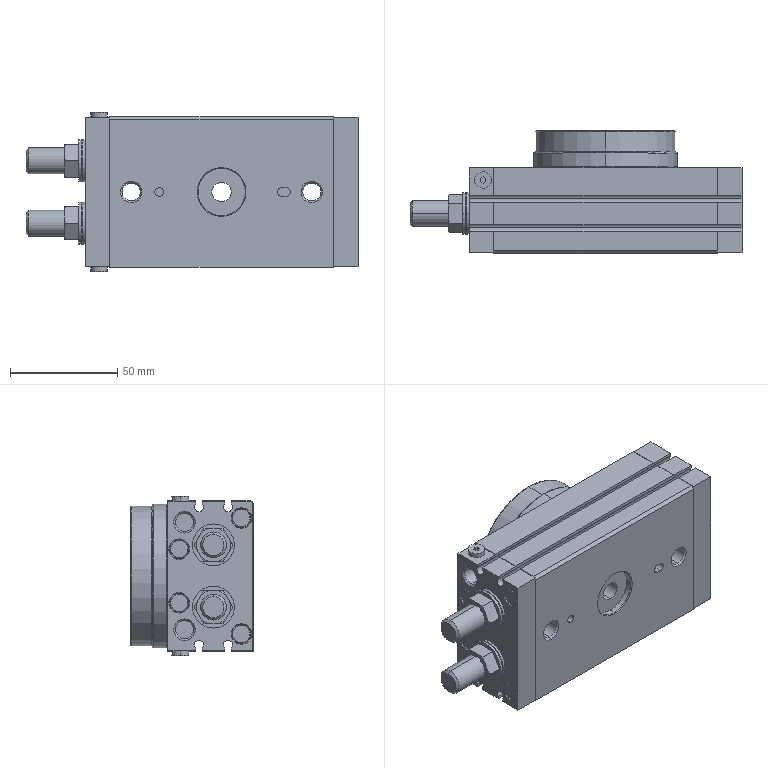Part | SolidWorks | 1 solid | 450 faces | box 154.5 x 57 x 74 mm | volume 391417 mm3 | cylinder 154 | plane 148 | cone 126 | spline 22 | commonest cylinder face diameters 4.917 x24 8.5 x20 9 x18 2.622 x12 4 x12 7.78 x12